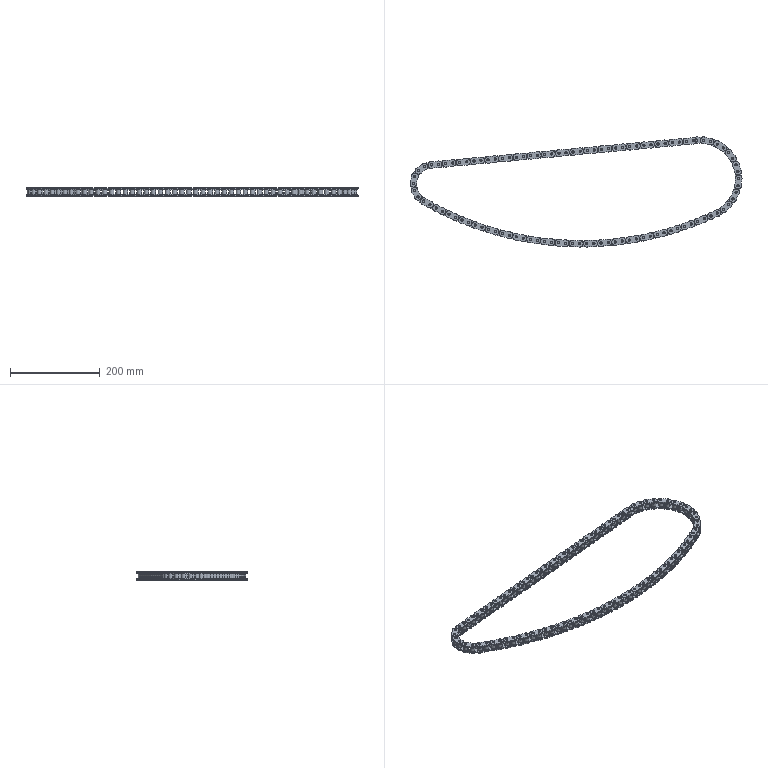Part | SolidWorks | features Boss 3, CurvePattern 2, Chamfer 1, CompositeCurve 1, Extrusion 1, MirrorPattern 1, MirrorSolid 1 | 153 solids | 3060 faces | volume 264927 mm3 | cylinder 2040 | plane 612 | cone 408 | commonest cylinder face diameters 5.09 x816 15.09 x612 69.169 x408 10.16 x204